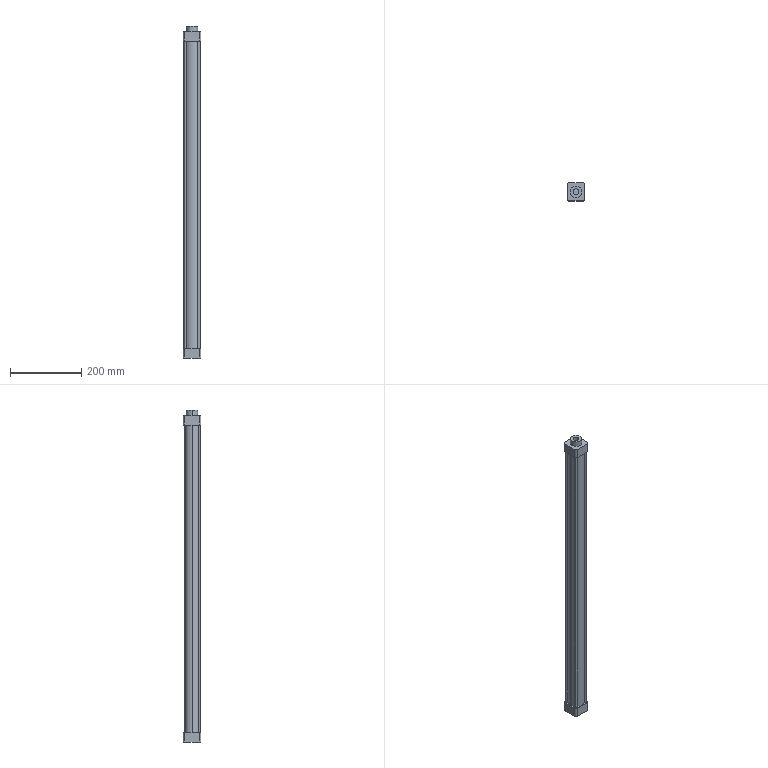Part | SolidWorks | features ICE 5, Extrusion 1, Fillet 1 | 1 solid | 39 faces | box 50 x 50 x 930 mm | volume 585630 mm3 | cylinder 24 | plane 15 | commonest cylinder face diameters 6 x8 10 x8 16 x2 32 x2 40 x2 46 x2
STEP:
#1=CARTESIAN_POINT('',(-15.5,-18.5,27.5));
#2=VERTEX_POINT('',#1);
#3=CARTESIAN_POINT('',(-21.5,-18.5,27.5));
#4=VERTEX_POINT('',#3);
#5=CARTESIAN_POINT('',(-18.5,-18.5,27.5));
#6=DIRECTION('',(0.,0.,1.));
#7=DIRECTION('',(1.,0.,0.));
#8=AXIS2_PLACEMENT_3D('',#5,#6,#7);
#9=CIRCLE('',#8,3.);
#10=EDGE_CURVE('',#2,#4,#9,.T.);
#11=ORIENTED_EDGE('',*,*,#10,.T.);
#12=CARTESIAN_POINT('',(-21.5,-18.5,887.5));
#13=VERTEX_POINT('',#12);
#14=CARTESIAN_POINT('',(-21.5,-18.5,-8.485));
#15=DIRECTION('',(0.,0.,1.));
#16=VECTOR('',#15,1000.);
#17=LINE('',#14,#16);
#18=EDGE_CURVE('',#4,#13,#17,.T.);
#19=ORIENTED_EDGE('',*,*,#18,.T.);
#20=CARTESIAN_POINT('',(-15.5,-18.5,887.5));
#21=VERTEX_POINT('',#20);
#22=CARTESIAN_POINT('',(-18.5,-18.5,887.5));
#23=DIRECTION('',(0.,0.,1.));
#24=DIRECTION('',(1.,0.,0.));
#25=AXIS2_PLACEMENT_3D('',#22,#23,#24);
#26=CIRCLE('',#25,3.);
#27=EDGE_CURVE('',#21,#13,#26,.T.);
#28=ORIENTED_EDGE('',*,*,#27,.F.);
#29=CARTESIAN_POINT('',(-15.5,-18.5,-8.485));
#30=DIRECTION('',(0.,0.,1.));
#31=VECTOR('',#30,1000.);
#32=LINE('',#29,#31);
#33=EDGE_CURVE('',#2,#21,#32,.T.);
#34=ORIENTED_EDGE('',*,*,#33,.F.);
#35=EDGE_LOOP('',(#11,#19,#28,#34));
#36=FACE_OUTER_BOUND('',#35,.T.);
#37=CARTESIAN_POINT('',(-18.5,-18.5,-8.485));
#38=DIRECTION('',(0.,0.,1.));
#39=DIRECTION('',(1.,0.,0.));
#40=AXIS2_PLACEMENT_3D('',#37,#38,#39);
#41=CYLINDRICAL_SURFACE('',#40,3.);
#42=ADVANCED_FACE('',(#36),#41,.T.);
#43=CARTESIAN_POINT('',(21.5,-18.5,27.5));
#44=VERTEX_POINT('',#43);
#45=CARTESIAN_POINT('',(15.5,-18.5,27.5));
#46=VERTEX_POINT('',#45);
#47=CARTESIAN_POINT('',(18.5,-18.5,27.5));
#48=DIRECTION('',(0.,0.,1.));
#49=DIRECTION('',(1.,0.,0.));
#50=AXIS2_PLACEMENT_3D('',#47,#48,#49);
#51=CIRCLE('',#50,3.);
#52=EDGE_CURVE('',#44,#46,#51,.T.);
#53=ORIENTED_EDGE('',*,*,#52,.T.);
#54=CARTESIAN_POINT('',(15.5,-18.5,887.5));
#55=VERTEX_POINT('',#54);
#56=CARTESIAN_POINT('',(15.5,-18.5,-8.485));
#57=DIRECTION('',(0.,0.,1.));
#58=VECTOR('',#57,1000.);
#59=LINE('',#56,#58);
#60=EDGE_CURVE('',#46,#55,#59,.T.);
#61=ORIENTED_EDGE('',*,*,#60,.T.);
#62=CARTESIAN_POINT('',(21.5,-18.5,887.5));
#63=VERTEX_POINT('',#62);
#64=CARTESIAN_POINT('',(18.5,-18.5,887.5));
#65=DIRECTION('',(0.,0.,1.));
#66=DIRECTION('',(1.,0.,0.));
#67=AXIS2_PLACEMENT_3D('',#64,#65,#66);
#68=CIRCLE('',#67,3.);
#69=EDGE_CURVE('',#63,#55,#68,.T.);
#70=ORIENTED_EDGE('',*,*,#69,.F.);
#71=CARTESIAN_POINT('',(21.5,-18.5,-8.485));
#72=DIRECTION('',(0.,0.,1.));
#73=VECTOR('',#72,1000.);
#74=LINE('',#71,#73);
#75=EDGE_CURVE('',#44,#63,#74,.T.);
#76=ORIENTED_EDGE('',*,*,#75,.F.);
#77=EDGE_LOOP('',(#53,#61,#70,#76));
#78=FACE_OUTER_BOUND('',#77,.T.);
#79=CARTESIAN_POINT('',(18.5,-18.5,-8.485));
#80=DIRECTION('',(0.,0.,1.));
#81=DIRECTION('',(1.,0.,0.));
#82=AXIS2_PLACEMENT_3D('',#79,#80,#81);
#83=CYLINDRICAL_SURFACE('',#82,3.);
#84=ADVANCED_FACE('',(#78),#83,.T.);
#85=CARTESIAN_POINT('',(21.5,18.5,27.5));
#86=VERTEX_POINT('',#85);
#87=CARTESIAN_POINT('',(15.5,18.5,27.5));
#88=VERTEX_POINT('',#87);
#89=CARTESIAN_POINT('',(18.5,18.5,27.5));
#90=DIRECTION('',(0.,0.,1.));
#91=DIRECTION('',(1.,0.,0.));
#92=AXIS2_PLACEMENT_3D('',#89,#90,#91);
#93=CIRCLE('',#92,3.);
#94=EDGE_CURVE('',#86,#88,#93,.T.);
#95=ORIENTED_EDGE('',*,*,#94,.T.);
#96=CARTESIAN_POINT('',(15.5,18.5,887.5));
#97=VERTEX_POINT('',#96);
#98=CARTESIAN_POINT('',(15.5,18.5,-8.485));
#99=DIRECTION('',(0.,0.,1.));
#100=VECTOR('',#99,1000.);
#101=LINE('',#98,#100);
#102=EDGE_CURVE('',#88,#97,#101,.T.);
#103=ORIENTED_EDGE('',*,*,#102,.T.);
#104=CARTESIAN_POINT('',(21.5,18.5,887.5));
#105=VERTEX_POINT('',#104);
#106=CARTESIAN_POINT('',(18.5,18.5,887.5));
#107=DIRECTION('',(0.,0.,1.));
#108=DIRECTION('',(1.,0.,0.));
#109=AXIS2_PLACEMENT_3D('',#106,#107,#108);
#110=CIRCLE('',#109,3.);
#111=EDGE_CURVE('',#105,#97,#110,.T.);
#112=ORIENTED_EDGE('',*,*,#111,.F.);
#113=CARTESIAN_POINT('',(21.5,18.5,-8.485));
#114=DIRECTION('',(0.,0.,1.));
#115=VECTOR('',#114,1000.);
#116=LINE('',#113,#115);
#117=EDGE_CURVE('',#86,#105,#116,.T.);
#118=ORIENTED_EDGE('',*,*,#117,.F.);
#119=EDGE_LOOP('',(#95,#103,#112,#118));
#120=FACE_OUTER_BOUND('',#119,.T.);
#121=CARTESIAN_POINT('',(18.5,18.5,-8.485));
#122=DIRECTION('',(0.,0.,1.));
#123=DIRECTION('',(1.,0.,0.));
#124=AXIS2_PLACEMENT_3D('',#121,#122,#123);
#125=CYLINDRICAL_SURFACE('',#124,3.);
#126=ADVANCED_FACE('',(#120),#125,.T.);
#127=CARTESIAN_POINT('',(-15.5,18.5,27.5));
#128=VERTEX_POINT('',#127);
#129=CARTESIAN_POINT('',(-21.5,18.5,27.5));
#130=VERTEX_POINT('',#129);
#131=CARTESIAN_POINT('',(-18.5,18.5,27.5));
#132=DIRECTION('',(0.,0.,1.));
#133=DIRECTION('',(1.,0.,0.));
#134=AXIS2_PLACEMENT_3D('',#131,#132,#133);
#135=CIRCLE('',#134,3.);
#136=EDGE_CURVE('',#128,#130,#135,.T.);
#137=ORIENTED_EDGE('',*,*,#136,.T.);
#138=CARTESIAN_POINT('',(-21.5,18.5,887.5));
#139=VERTEX_POINT('',#138);
#140=CARTESIAN_POINT('',(-21.5,18.5,-8.485));
#141=DIRECTION('',(0.,0.,1.));
#142=VECTOR('',#141,1000.);
#143=LINE('',#140,#142);
#144=EDGE_CURVE('',#130,#139,#143,.T.);
#145=ORIENTED_EDGE('',*,*,#144,.T.);
#146=CARTESIAN_POINT('',(-15.5,18.5,887.5));
#147=VERTEX_POINT('',#146);
#148=CARTESIAN_POINT('',(-18.5,18.5,887.5));
#149=DIRECTION('',(0.,0.,1.));
#150=DIRECTION('',(1.,0.,0.));
#151=AXIS2_PLACEMENT_3D('',#148,#149,#150);
#152=CIRCLE('',#151,3.);
#153=EDGE_CURVE('',#147,#139,#152,.T.);
#154=ORIENTED_EDGE('',*,*,#153,.F.);
#155=CARTESIAN_POINT('',(-15.5,18.5,-8.485));
#156=DIRECTION('',(0.,0.,1.));
#157=VECTOR('',#156,1000.);
#158=LINE('',#155,#157);
#159=EDGE_CURVE('',#128,#147,#158,.T.);
#160=ORIENTED_EDGE('',*,*,#159,.F.);
#161=EDGE_LOOP('',(#137,#145,#154,#160));
#162=FACE_OUTER_BOUND('',#161,.T.);
#163=CARTESIAN_POINT('',(-18.5,18.5,-8.485));
#164=DIRECTION('',(0.,0.,1.));
#165=DIRECTION('',(1.,0.,0.));
#166=AXIS2_PLACEMENT_3D('',#163,#164,#165);
#167=CYLINDRICAL_SURFACE('',#166,3.);
#168=ADVANCED_FACE('',(#162),#167,.T.);
#169=CARTESIAN_POINT('',(16.,0.,930.));
#170=VERTEX_POINT('',#169);
#171=CARTESIAN_POINT('',(-16.,0.,930.));
#172=VERTEX_POINT('',#171);
#173=CARTESIAN_POINT('',(0.,0.,930.));
#174=DIRECTION('',(0.,0.,1.));
#175=DIRECTION('',(1.,0.,0.));
#176=AXIS2_PLACEMENT_3D('',#173,#174,#175);
#177=CIRCLE('',#176,16.);
#178=EDGE_CURVE('',#170,#172,#177,.T.);
#179=ORIENTED_EDGE('',*,*,#178,.F.);
#180=CARTESIAN_POINT('',(16.,0.,915.));
#181=VERTEX_POINT('',#180);
#182=CARTESIAN_POINT('',(16.,0.,930.));
#183=DIRECTION('',(0.,0.,-1.));
#184=VECTOR('',#183,1000.);
#185=LINE('',#182,#184);
#186=EDGE_CURVE('',#170,#181,#185,.T.);
#187=ORIENTED_EDGE('',*,*,#186,.T.);
#188=CARTESIAN_POINT('',(-16.,0.,915.));
#189=VERTEX_POINT('',#188);
#190=CARTESIAN_POINT('',(0.,0.,915.));
#191=DIRECTION('',(0.,0.,1.));
#192=DIRECTION('',(1.,0.,0.));
#193=AXIS2_PLACEMENT_3D('',#190,#191,#192);
#194=CIRCLE('',#193,16.);
#195=EDGE_CURVE('',#181,#189,#194,.T.);
#196=ORIENTED_EDGE('',*,*,#195,.T.);
#197=CARTESIAN_POINT('',(-16.,0.,930.));
#198=DIRECTION('',(0.,0.,-1.));
#199=VECTOR('',#198,1000.);
#200=LINE('',#197,#199);
#201=EDGE_CURVE('',#172,#189,#200,.T.);
#202=ORIENTED_EDGE('',*,*,#201,.F.);
#203=EDGE_LOOP('',(#179,#187,#196,#202));
#204=FACE_OUTER_BOUND('',#203,.T.);
#205=CARTESIAN_POINT('',(0.,0.,930.));
#206=DIRECTION('',(0.,0.,-1.));
#207=DIRECTION('',(-1.,0.,0.));
#208=AXIS2_PLACEMENT_3D('',#205,#206,#207);
#209=CYLINDRICAL_SURFACE('',#208,16.);
#210=ADVANCED_FACE('',(#204),#209,.T.);
#211=CARTESIAN_POINT('',(23.,0.,887.5));
#212=VERTEX_POINT('',#211);
#213=CARTESIAN_POINT('',(-23.,0.,887.5));
#214=VERTEX_POINT('',#213);
#215=CARTESIAN_POINT('',(0.,0.,887.5));
#216=DIRECTION('',(0.,0.,1.));
#217=DIRECTION('',(1.,0.,0.));
#218=AXIS2_PLACEMENT_3D('',#215,#216,#217);
#219=CIRCLE('',#218,23.);
#220=EDGE_CURVE('',#212,#214,#219,.T.);
#221=ORIENTED_EDGE('',*,*,#220,.F.);
#222=CARTESIAN_POINT('',(23.,0.,27.5));
#223=VERTEX_POINT('',#222);
#224=CARTESIAN_POINT('',(23.,0.,887.5));
#225=DIRECTION('',(0.,0.,-1.));
#226=VECTOR('',#225,1000.);
#227=LINE('',#224,#226);
#228=EDGE_CURVE('',#212,#223,#227,.T.);
#229=ORIENTED_EDGE('',*,*,#228,.T.);
#230=CARTESIAN_POINT('',(-23.,0.,27.5));
#231=VERTEX_POINT('',#230);
#232=CARTESIAN_POINT('',(0.,0.,27.5));
#233=DIRECTION('',(0.,0.,1.));
#234=DIRECTION('',(1.,0.,0.));
#235=AXIS2_PLACEMENT_3D('',#232,#233,#234);
#236=CIRCLE('',#235,23.);
#237=EDGE_CURVE('',#223,#231,#236,.T.);
#238=ORIENTED_EDGE('',*,*,#237,.T.);
#239=CARTESIAN_POINT('',(-23.,0.,887.5));
#240=DIRECTION('',(0.,0.,-1.));
#241=VECTOR('',#240,1000.);
#242=LINE('',#239,#241);
#243=EDGE_CURVE('',#214,#231,#242,.T.);
#244=ORIENTED_EDGE('',*,*,#243,.F.);
#245=EDGE_LOOP('',(#221,#229,#238,#244));
#246=FACE_OUTER_BOUND('',#245,.T.);
#247=CARTESIAN_POINT('',(0.,0.,887.5));
#248=DIRECTION('',(0.,0.,-1.));
#249=DIRECTION('',(-1.,0.,0.));
#250=AXIS2_PLACEMENT_3D('',#247,#248,#249);
#251=CYLINDRICAL_SURFACE('',#250,23.);
#252=ADVANCED_FACE('',(#246),#251,.T.);
#253=CARTESIAN_POINT('',(-8.,0.,887.5));
#254=VERTEX_POINT('',#253);
#255=CARTESIAN_POINT('',(8.,0.,887.5));
#256=VERTEX_POINT('',#255);
#257=CARTESIAN_POINT('',(0.,0.,887.5));
#258=DIRECTION('',(0.,0.,1.));
#259=DIRECTION('',(1.,0.,0.));
#260=AXIS2_PLACEMENT_3D('',#257,#258,#259);
#261=CIRCLE('',#260,8.);
#262=EDGE_CURVE('',#254,#256,#261,.T.);
#263=ORIENTED_EDGE('',*,*,#262,.F.);
#264=CARTESIAN_POINT('',(-8.,0.,930.));
#265=VERTEX_POINT('',#264);
#266=CARTESIAN_POINT('',(-8.,0.,830.));
#267=DIRECTION('',(0.,0.,1.));
#268=VECTOR('',#267,1000.);
#269=LINE('',#266,#268);
#270=EDGE_CURVE('',#254,#265,#269,.T.);
#271=ORIENTED_EDGE('',*,*,#270,.T.);
#272=CARTESIAN_POINT('',(8.,0.,930.));
#273=VERTEX_POINT('',#272);
#274=CARTESIAN_POINT('',(0.,0.,930.));
#275=DIRECTION('',(0.,0.,1.));
#276=DIRECTION('',(1.,0.,0.));
#277=AXIS2_PLACEMENT_3D('',#274,#275,#276);
#278=CIRCLE('',#277,8.);
#279=EDGE_CURVE('',#265,#273,#278,.T.);
#280=ORIENTED_EDGE('',*,*,#279,.T.);
#281=CARTESIAN_POINT('',(8.,0.,830.));
#282=DIRECTION('',(0.,0.,1.));
#283=VECTOR('',#282,1000.);
#284=LINE('',#281,#283);
#285=EDGE_CURVE('',#256,#273,#284,.T.);
#286=ORIENTED_EDGE('',*,*,#285,.F.);
#287=EDGE_LOOP('',(#263,#271,#280,#286));
#288=FACE_OUTER_BOUND('',#287,.T.);
#289=CARTESIAN_POINT('',(0.,0.,830.));
#290=DIRECTION('',(0.,0.,1.));
#291=DIRECTION('',(1.,0.,0.));
#292=AXIS2_PLACEMENT_3D('',#289,#290,#291);
#293=CYLINDRICAL_SURFACE('',#292,8.);
#294=ADVANCED_FACE('',(#288),#293,.F.);
#295=CARTESIAN_POINT('',(-20.,0.,887.5));
#296=VERTEX_POINT('',#295);
#297=CARTESIAN_POINT('',(20.,0.,887.5));
#298=VERTEX_POINT('',#297);
#299=CARTESIAN_POINT('',(0.,0.,887.5));
#300=DIRECTION('',(0.,0.,1.));
#301=DIRECTION('',(1.,0.,0.));
#302=AXIS2_PLACEMENT_3D('',#299,#300,#301);
#303=CIRCLE('',#302,20.);
#304=EDGE_CURVE('',#296,#298,#303,.T.);
#305=ORIENTED_EDGE('',*,*,#304,.T.);
#306=CARTESIAN_POINT('',(20.,0.,27.5));
#307=VERTEX_POINT('',#306);
#308=CARTESIAN_POINT('',(20.,0.,887.5));
#309=DIRECTION('',(0.,0.,-1.));
#310=VECTOR('',#309,1000.);
#311=LINE('',#308,#310);
#312=EDGE_CURVE('',#298,#307,#311,.T.);
#313=ORIENTED_EDGE('',*,*,#312,.T.);
#314=CARTESIAN_POINT('',(-20.,0.,27.5));
#315=VERTEX_POINT('',#314);
#316=CARTESIAN_POINT('',(0.,0.,27.5));
#317=DIRECTION('',(0.,0.,-1.));
#318=DIRECTION('',(1.,0.,0.));
#319=AXIS2_PLACEMENT_3D('',#316,#317,#318);
#320=CIRCLE('',#319,20.);
#321=EDGE_CURVE('',#307,#315,#320,.T.);
#322=ORIENTED_EDGE('',*,*,#321,.T.);
#323=CARTESIAN_POINT('',(-20.,0.,887.5));
#324=DIRECTION('',(0.,0.,-1.));
#325=VECTOR('',#324,1000.);
#326=LINE('',#323,#325);
#327=EDGE_CURVE('',#296,#315,#326,.T.);
#328=ORIENTED_EDGE('',*,*,#327,.F.);
#329=EDGE_LOOP('',(#305,#313,#322,#328));
#330=FACE_OUTER_BOUND('',#329,.T.);
#331=CARTESIAN_POINT('',(0.,0.,887.5));
#332=DIRECTION('',(0.,0.,-1.));
#333=DIRECTION('',(-1.,0.,0.));
#334=AXIS2_PLACEMENT_3D('',#331,#332,#333);
#335=CYLINDRICAL_SURFACE('',#334,20.);
#336=ADVANCED_FACE('',(#330),#335,.F.);
#337=CARTESIAN_POINT('',(0.,0.,27.5));
#338=DIRECTION('',(0.,0.,-1.));
#339=DIRECTION('',(1.,0.,0.));
#340=AXIS2_PLACEMENT_3D('',#337,#338,#339);
#341=CIRCLE('',#340,20.);
#342=EDGE_CURVE('',#315,#307,#341,.T.);
#343=ORIENTED_EDGE('',*,*,#342,.F.);
#344=ORIENTED_EDGE('',*,*,#321,.F.);
#345=EDGE_LOOP('',(#343,#344));
#346=FACE_OUTER_BOUND('',#345,.T.);
#347=CARTESIAN_POINT('',(0.,0.,27.5));
#348=DIRECTION('',(0.,0.,1.));
#349=DIRECTION('',(1.,0.,0.));
#350=AXIS2_PLACEMENT_3D('',#347,#348,#349);
#351=PLANE('',#350);
#352=ADVANCED_FACE('',(#346),#351,.T.);
#353=ORIENTED_EDGE('',*,*,#312,.F.);
#354=CARTESIAN_POINT('',(0.,0.,887.5));
#355=DIRECTION('',(0.,0.,1.));
#356=DIRECTION('',(1.,0.,0.));
#357=AXIS2_PLACEMENT_3D('',#354,#355,#356);
#358=CIRCLE('',#357,20.);
#359=EDGE_CURVE('',#298,#296,#358,.T.);
#360=ORIENTED_EDGE('',*,*,#359,.T.);
#361=ORIENTED_EDGE('',*,*,#327,.T.);
#362=ORIENTED_EDGE('',*,*,#342,.T.);
#363=EDGE_LOOP('',(#353,#360,#361,#362));
#364=FACE_OUTER_BOUND('',#363,.T.);
#365=CARTESIAN_POINT('',(0.,0.,887.5));
#366=DIRECTION('',(0.,0.,-1.));
#367=DIRECTION('',(-1.,0.,0.));
#368=AXIS2_PLACEMENT_3D('',#365,#366,#367);
#369=CYLINDRICAL_SURFACE('',#368,20.);
#370=ADVANCED_FACE('',(#364),#369,.F.);
#371=CARTESIAN_POINT('',(0.,0.,887.5));
#372=DIRECTION('',(0.,0.,1.));
#373=DIRECTION('',(1.,0.,0.));
#374=AXIS2_PLACEMENT_3D('',#371,#372,#373);
#375=CIRCLE('',#374,8.);
#376=EDGE_CURVE('',#256,#254,#375,.T.);
#377=ORIENTED_EDGE('',*,*,#376,.T.);
#378=ORIENTED_EDGE('',*,*,#262,.T.);
#379=EDGE_LOOP('',(#377,#378));
#380=FACE_BOUND('',#379,.T.);
#381=ORIENTED_EDGE('',*,*,#304,.F.);
#382=ORIENTED_EDGE('',*,*,#359,.F.);
#383=EDGE_LOOP('',(#381,#382));
#384=FACE_OUTER_BOUND('',#383,.T.);
#385=CARTESIAN_POINT('',(0.,0.,887.5));
#386=DIRECTION('',(0.,0.,1.));
#387=DIRECTION('',(1.,0.,0.));
#388=AXIS2_PLACEMENT_3D('',#385,#386,#387);
#389=PLANE('',#388);
#390=ADVANCED_FACE('',(#380,#384),#389,.F.);
#391=ORIENTED_EDGE('',*,*,#270,.F.);
#392=ORIENTED_EDGE('',*,*,#376,.F.);
#393=ORIENTED_EDGE('',*,*,#285,.T.);
#394=CARTESIAN_POINT('',(0.,0.,930.));
#395=DIRECTION('',(0.,0.,1.));
#396=DIRECTION('',(1.,0.,0.));
#397=AXIS2_PLACEMENT_3D('',#394,#395,#396);
#398=CIRCLE('',#397,8.);
#399=EDGE_CURVE('',#273,#265,#398,.T.);
#400=ORIENTED_EDGE('',*,*,#399,.T.);
#401=EDGE_LOOP('',(#391,#392,#393,#400));
#402=FACE_OUTER_BOUND('',#401,.T.);
#403=CARTESIAN_POINT('',(0.,0.,830.));
#404=DIRECTION('',(0.,0.,1.));
#405=DIRECTION('',(1.,0.,0.));
#406=AXIS2_PLACEMENT_3D('',#403,#404,#405);
#407=CYLINDRICAL_SURFACE('',#406,8.);
#408=ADVANCED_FACE('',(#402),#407,.F.);
#409=CARTESIAN_POINT('',(25.,-20.,27.5));
#410=VERTEX_POINT('',#409);
#411=CARTESIAN_POINT('',(25.,20.,27.5));
#412=VERTEX_POINT('',#411);
#413=CARTESIAN_POINT('',(25.,25.,27.5));
#414=DIRECTION('',(0.,1.,0.));
#415=VECTOR('',#414,1000.);
#416=LINE('',#413,#415);
#417=EDGE_CURVE('',#410,#412,#416,.T.);
#418=ORIENTED_EDGE('',*,*,#417,.F.);
#419=CARTESIAN_POINT('',(25.,-20.,0.));
#420=VERTEX_POINT('',#419);
#421=CARTESIAN_POINT('',(25.,-20.,27.5));
#422=DIRECTION('',(0.,0.,-1.));
#423=VECTOR('',#422,1000.);
#424=LINE('',#421,#423);
#425=EDGE_CURVE('',#410,#420,#424,.T.);
#426=ORIENTED_EDGE('',*,*,#425,.T.);
#427=CARTESIAN_POINT('',(25.,20.,0.));
#428=VERTEX_POINT('',#427);
#429=CARTESIAN_POINT('',(25.,25.,0.));
#430=DIRECTION('',(0.,1.,0.));
#431=VECTOR('',#430,1000.);
#432=LINE('',#429,#431);
#433=EDGE_CURVE('',#420,#428,#432,.T.);
#434=ORIENTED_EDGE('',*,*,#433,.T.);
#435=CARTESIAN_POINT('',(25.,20.,27.5));
#436=DIRECTION('',(0.,0.,1.));
#437=VECTOR('',#436,1000.);
#438=LINE('',#435,#437);
#439=EDGE_CURVE('',#428,#412,#438,.T.);
#440=ORIENTED_EDGE('',*,*,#439,.T.);
#441=EDGE_LOOP('',(#418,#426,#434,#440));
#442=FACE_OUTER_BOUND('',#441,.T.);
#443=CARTESIAN_POINT('',(25.,25.,27.5));
#444=DIRECTION('',(-1.,0.,0.));
#445=DIRECTION('',(0.,0.,1.));
#446=AXIS2_PLACEMENT_3D('',#443,#444,#445);
#447=PLANE('',#446);
#448=ADVANCED_FACE('',(#442),#447,.F.);
#449=CARTESIAN_POINT('',(20.,25.,0.));
#450=VERTEX_POINT('',#449);
#451=CARTESIAN_POINT('',(-20.,25.,0.));
#452=VERTEX_POINT('',#451);
#453=CARTESIAN_POINT('',(-25.,25.,0.));
#454=DIRECTION('',(-1.,0.,0.));
#455=VECTOR('',#454,1000.);
#456=LINE('',#453,#455);
#457=EDGE_CURVE('',#450,#452,#456,.T.);
#458=ORIENTED_EDGE('',*,*,#457,.T.);
#459=CARTESIAN_POINT('',(-20.,25.,27.5));
#460=VERTEX_POINT('',#459);
#461=CARTESIAN_POINT('',(-20.,25.,27.5));
#462=DIRECTION('',(0.,0.,1.));
#463=VECTOR('',#462,1000.);
#464=LINE('',#461,#463);
#465=EDGE_CURVE('',#452,#460,#464,.T.);
#466=ORIENTED_EDGE('',*,*,#465,.T.);
#467=CARTESIAN_POINT('',(20.,25.,27.5));
#468=VERTEX_POINT('',#467);
#469=CARTESIAN_POINT('',(-25.,25.,27.5));
#470=DIRECTION('',(-1.,0.,0.));
#471=VECTOR('',#470,1000.);
#472=LINE('',#469,#471);
#473=EDGE_CURVE('',#468,#460,#472,.T.);
#474=ORIENTED_EDGE('',*,*,#473,.F.);
#475=CARTESIAN_POINT('',(20.,25.,27.5));
#476=DIRECTION('',(0.,0.,-1.));
#477=VECTOR('',#476,1000.);
#478=LINE('',#475,#477);
#479=EDGE_CURVE('',#468,#450,#478,.T.);
#480=ORIENTED_EDGE('',*,*,#479,.T.);
#481=EDGE_LOOP('',(#458,#466,#474,#480));
#482=FACE_OUTER_BOUND('',#481,.T.);
#483=CARTESIAN_POINT('',(-25.,25.,27.5));
#484=DIRECTION('',(0.,-1.,0.));
#485=DIRECTION('',(0.,0.,-1.));
#486=AXIS2_PLACEMENT_3D('',#483,#484,#485);
#487=PLANE('',#486);
#488=ADVANCED_FACE('',(#482),#487,.F.);
#489=CARTESIAN_POINT('',(-25.,20.,0.));
#490=VERTEX_POINT('',#489);
#491=CARTESIAN_POINT('',(-25.,-20.,0.));
#492=VERTEX_POINT('',#491);
#493=CARTESIAN_POINT('',(-25.,25.,0.));
#494=DIRECTION('',(0.,-1.,0.));
#495=VECTOR('',#494,1000.);
#496=LINE('',#493,#495);
#497=EDGE_CURVE('',#490,#492,#496,.T.);
#498=ORIENTED_EDGE('',*,*,#497,.T.);
#499=CARTESIAN_POINT('',(-25.,-20.,27.5));
#500=VERTEX_POINT('',#499);
#501=CARTESIAN_POINT('',(-25.,-20.,27.5));
#502=DIRECTION('',(0.,0.,1.));
#503=VECTOR('',#502,1000.);
#504=LINE('',#501,#503);
#505=EDGE_CURVE('',#492,#500,#504,.T.);
#506=ORIENTED_EDGE('',*,*,#505,.T.);
#507=CARTESIAN_POINT('',(-25.,20.,27.5));
#508=VERTEX_POINT('',#507);
#509=CARTESIAN_POINT('',(-25.,25.,27.5));
#510=DIRECTION('',(0.,-1.,0.));
#511=VECTOR('',#510,1000.);
#512=LINE('',#509,#511);
#513=EDGE_CURVE('',#508,#500,#512,.T.);
#514=ORIENTED_EDGE('',*,*,#513,.F.);
#515=CARTESIAN_POINT('',(-25.,20.,27.5));
#516=DIRECTION('',(0.,0.,-1.));
#517=VECTOR('',#516,1000.);
#518=LINE('',#515,#517);
#519=EDGE_CURVE('',#508,#490,#518,.T.);
#520=ORIENTED_EDGE('',*,*,#519,.T.);
#521=EDGE_LOOP('',(#498,#506,#514,#520));
#522=FACE_OUTER_BOUND('',#521,.T.);
#523=CARTESIAN_POINT('',(-25.,25.,27.5));
#524=DIRECTION('',(1.,0.,0.));
#525=DIRECTION('',(0.,1.,0.));
#526=AXIS2_PLACEMENT_3D('',#523,#524,#525);
#527=PLANE('',#526);
#528=ADVANCED_FACE('',(#522),#527,.F.);
#529=CARTESIAN_POINT('',(-20.,-25.,27.5));
#530=VERTEX_POINT('',#529);
#531=CARTESIAN_POINT('',(20.,-25.,27.5));
#532=VERTEX_POINT('',#531);
#533=CARTESIAN_POINT('',(-25.,-25.,27.5));
#534=DIRECTION('',(1.,0.,0.));
#535=VECTOR('',#534,1000.);
#536=LINE('',#533,#535);
#537=EDGE_CURVE('',#530,#532,#536,.T.);
#538=ORIENTED_EDGE('',*,*,#537,.F.);
#539=CARTESIAN_POINT('',(-20.,-25.,0.));
#540=VERTEX_POINT('',#539);
#541=CARTESIAN_POINT('',(-20.,-25.,27.5));
#542=DIRECTION('',(0.,0.,-1.));
#543=VECTOR('',#542,1000.);
#544=LINE('',#541,#543);
#545=EDGE_CURVE('',#530,#540,#544,.T.);
#546=ORIENTED_EDGE('',*,*,#545,.T.);
#547=CARTESIAN_POINT('',(20.,-25.,0.));
#548=VERTEX_POINT('',#547);
#549=CARTESIAN_POINT('',(-25.,-25.,0.));
#550=DIRECTION('',(1.,0.,0.));
#551=VECTOR('',#550,1000.);
#552=LINE('',#549,#551);
#553=EDGE_CURVE('',#540,#548,#552,.T.);
#554=ORIENTED_EDGE('',*,*,#553,.T.);
#555=CARTESIAN_POINT('',(20.,-25.,27.5));
#556=DIRECTION('',(0.,0.,1.));
#557=VECTOR('',#556,1000.);
#558=LINE('',#555,#557);
#559=EDGE_CURVE('',#548,#532,#558,.T.);
#560=ORIENTED_EDGE('',*,*,#559,.T.);
#561=EDGE_LOOP('',(#538,#546,#554,#560));
#562=FACE_OUTER_BOUND('',#561,.T.);
#563=CARTESIAN_POINT('',(-25.,-25.,27.5));
#564=DIRECTION('',(0.,1.,0.));
#565=DIRECTION('',(0.,0.,1.));
#566=AXIS2_PLACEMENT_3D('',#563,#564,#565);
#567=PLANE('',#566);
#568=ADVANCED_FACE('',(#562),#567,.F.);
#569=ORIENTED_EDGE('',*,*,#10,.F.);
#570=CARTESIAN_POINT('',(-18.5,-18.5,27.5));
#571=DIRECTION('',(0.,0.,1.));
#572=DIRECTION('',(1.,0.,0.));
#573=AXIS2_PLACEMENT_3D('',#570,#571,#572);
#574=CIRCLE('',#573,3.);
#575=EDGE_CURVE('',#4,#2,#574,.T.);
#576=ORIENTED_EDGE('',*,*,#575,.F.);
#577=EDGE_LOOP('',(#569,#576));
#578=FACE_BOUND('',#577,.T.);
#579=ORIENTED_EDGE('',*,*,#52,.F.);
#580=CARTESIAN_POINT('',(18.5,-18.5,27.5));
#581=DIRECTION('',(0.,0.,1.));
#582=DIRECTION('',(1.,0.,0.));
#583=AXIS2_PLACEMENT_3D('',#580,#581,#582);
#584=CIRCLE('',#583,3.);
#585=EDGE_CURVE('',#46,#44,#584,.T.);
#586=ORIENTED_EDGE('',*,*,#585,.F.);
#587=EDGE_LOOP('',(#579,#586));
#588=FACE_BOUND('',#587,.T.);
#589=ORIENTED_EDGE('',*,*,#94,.F.);
#590=CARTESIAN_POINT('',(18.5,18.5,27.5));
#591=DIRECTION('',(0.,0.,1.));
#592=DIRECTION('',(1.,0.,0.));
#593=AXIS2_PLACEMENT_3D('',#590,#591,#592);
#594=CIRCLE('',#593,3.);
#595=EDGE_CURVE('',#88,#86,#594,.T.);
#596=ORIENTED_EDGE('',*,*,#595,.F.);
#597=EDGE_LOOP('',(#589,#596));
#598=FACE_BOUND('',#597,.T.);
#599=ORIENTED_EDGE('',*,*,#136,.F.);
#600=CARTESIAN_POINT('',(-18.5,18.5,27.5));
#601=DIRECTION('',(0.,0.,1.));
#602=DIRECTION('',(1.,0.,0.));
#603=AXIS2_PLACEMENT_3D('',#600,#601,#602);
#604=CIRCLE('',#603,3.);
#605=EDGE_CURVE('',#130,#128,#604,.T.);
#606=ORIENTED_EDGE('',*,*,#605,.F.);
#607=EDGE_LOOP('',(#599,#606));
#608=FACE_BOUND('',#607,.T.);
#609=CARTESIAN_POINT('',(0.,0.,27.5));
#610=DIRECTION('',(0.,0.,1.));
#611=DIRECTION('',(1.,0.,0.));
#612=AXIS2_PLACEMENT_3D('',#609,#610,#611);
#613=CIRCLE('',#612,23.);
#614=EDGE_CURVE('',#231,#223,#613,.T.);
#615=ORIENTED_EDGE('',*,*,#614,.F.);
#616=ORIENTED_EDGE('',*,*,#237,.F.);
#617=EDGE_LOOP('',(#615,#616));
#618=FACE_BOUND('',#617,.T.);
#619=ORIENTED_EDGE('',*,*,#513,.T.);
#620=CARTESIAN_POINT('',(-20.,-20.,27.5));
#621=DIRECTION('',(0.,0.,1.));
#622=DIRECTION('',(1.,0.,0.));
#623=AXIS2_PLACEMENT_3D('',#620,#621,#622);
#624=CIRCLE('',#623,5.);
#625=EDGE_CURVE('',#500,#530,#624,.T.);
#626=ORIENTED_EDGE('',*,*,#625,.T.);
#627=ORIENTED_EDGE('',*,*,#537,.T.);
#628=CARTESIAN_POINT('',(20.,-20.,27.5));
#629=DIRECTION('',(0.,0.,1.));
#630=DIRECTION('',(1.,0.,0.));
#631=AXIS2_PLACEMENT_3D('',#628,#629,#630);
#632=CIRCLE('',#631,5.);
#633=EDGE_CURVE('',#532,#410,#632,.T.);
#634=ORIENTED_EDGE('',*,*,#633,.T.);
#635=ORIENTED_EDGE('',*,*,#417,.T.);
#636=CARTESIAN_POINT('',(20.,20.,27.5));
#637=DIRECTION('',(0.,0.,1.));
#638=DIRECTION('',(1.,0.,0.));
#639=AXIS2_PLACEMENT_3D('',#636,#637,#638);
#640=CIRCLE('',#639,5.);
#641=EDGE_CURVE('',#412,#468,#640,.T.);
#642=ORIENTED_EDGE('',*,*,#641,.T.);
#643=ORIENTED_EDGE('',*,*,#473,.T.);
#644=CARTESIAN_POINT('',(-20.,20.,27.5));
#645=DIRECTION('',(0.,0.,1.));
#646=DIRECTION('',(1.,0.,0.));
#647=AXIS2_PLACEMENT_3D('',#644,#645,#646);
#648=CIRCLE('',#647,5.);
#649=EDGE_CURVE('',#460,#508,#648,.T.);
#650=ORIENTED_EDGE('',*,*,#649,.T.);
#651=EDGE_LOOP('',(#619,#626,#627,#634,#635,#642,#643,#650));
#652=FACE_OUTER_BOUND('',#651,.T.);
#653=CARTESIAN_POINT('',(0.,0.,27.5));
#654=DIRECTION('',(0.,0.,1.));
#655=DIRECTION('',(1.,0.,0.));
#656=AXIS2_PLACEMENT_3D('',#653,#654,#655);
#657=PLANE('',#656);
#658=ADVANCED_FACE('',(#578,#588,#598,#608,#618,#652),#657,.T.);
#659=ORIENTED_EDGE('',*,*,#553,.F.);
#660=CARTESIAN_POINT('',(-20.,-20.,0.));
#661=DIRECTION('',(0.,0.,-1.));
#662=DIRECTION('',(1.,0.,0.));
#663=AXIS2_PLACEMENT_3D('',#660,#661,#662);
#664=CIRCLE('',#663,5.);
#665=EDGE_CURVE('',#540,#492,#664,.T.);
#666=ORIENTED_EDGE('',*,*,#665,.T.);
#667=ORIENTED_EDGE('',*,*,#497,.F.);
#668=CARTESIAN_POINT('',(-20.,20.,0.));
#669=DIRECTION('',(0.,0.,-1.));
#670=DIRECTION('',(1.,0.,0.));
#671=AXIS2_PLACEMENT_3D('',#668,#669,#670);
#672=CIRCLE('',#671,5.);
#673=EDGE_CURVE('',#490,#452,#672,.T.);
#674=ORIENTED_EDGE('',*,*,#673,.T.);
#675=ORIENTED_EDGE('',*,*,#457,.F.);
#676=CARTESIAN_POINT('',(20.,20.,0.));
#677=DIRECTION('',(0.,0.,-1.));
#678=DIRECTION('',(1.,0.,0.));
#679=AXIS2_PLACEMENT_3D('',#676,#677,#678);
#680=CIRCLE('',#679,5.);
#681=EDGE_CURVE('',#450,#428,#680,.T.);
#682=ORIENTED_EDGE('',*,*,#681,.T.);
#683=ORIENTED_EDGE('',*,*,#433,.F.);
#684=CARTESIAN_POINT('',(20.,-20.,0.));
#685=DIRECTION('',(0.,0.,-1.));
#686=DIRECTION('',(1.,0.,0.));
#687=AXIS2_PLACEMENT_3D('',#684,#685,#686);
#688=CIRCLE('',#687,5.);
#689=EDGE_CURVE('',#420,#548,#688,.T.);
#690=ORIENTED_EDGE('',*,*,#689,.T.);
#691=EDGE_LOOP('',(#659,#666,#667,#674,#675,#682,#683,#690));
#692=FACE_OUTER_BOUND('',#691,.T.);
#693=CARTESIAN_POINT('',(0.,0.,0.));
#694=DIRECTION('',(0.,0.,1.));
#695=DIRECTION('',(1.,0.,0.));
#696=AXIS2_PLACEMENT_3D('',#693,#694,#695);
#697=PLANE('',#696);
#698=ADVANCED_FACE('',(#692),#697,.F.);
#699=ORIENTED_EDGE('',*,*,#228,.F.);
#700=CARTESIAN_POINT('',(0.,0.,887.5));
#701=DIRECTION('',(0.,0.,1.));
#702=DIRECTION('',(1.,0.,0.));
#703=AXIS2_PLACEMENT_3D('',#700,#701,#702);
#704=CIRCLE('',#703,23.);
#705=EDGE_CURVE('',#214,#212,#704,.T.);
#706=ORIENTED_EDGE('',*,*,#705,.F.);
#707=ORIENTED_EDGE('',*,*,#243,.T.);
#708=ORIENTED_EDGE('',*,*,#614,.T.);
#709=EDGE_LOOP('',(#699,#706,#707,#708));
#710=FACE_OUTER_BOUND('',#709,.T.);
#711=CARTESIAN_POINT('',(0.,0.,887.5));
#712=DIRECTION('',(0.,0.,-1.));
#713=DIRECTION('',(-1.,0.,0.));
#714=AXIS2_PLACEMENT_3D('',#711,#712,#713);
#715=CYLINDRICAL_SURFACE('',#714,23.);
#716=ADVANCED_FACE('',(#710),#715,.T.);
#717=CARTESIAN_POINT('',(25.,-20.,915.));
#718=VERTEX_POINT('',#717);
#719=CARTESIAN_POINT('',(25.,20.,915.));
#720=VERTEX_POINT('',#719);
#721=CARTESIAN_POINT('',(25.,25.,915.));
#722=DIRECTION('',(0.,1.,0.));
#723=VECTOR('',#722,1000.);
#724=LINE('',#721,#723);
#725=EDGE_CURVE('',#718,#720,#724,.T.);
#726=ORIENTED_EDGE('',*,*,#725,.F.);
#727=CARTESIAN_POINT('',(25.,-20.,887.5));
#728=VERTEX_POINT('',#727);
#729=CARTESIAN_POINT('',(25.,-20.,915.));
#730=DIRECTION('',(0.,0.,-1.));
#731=VECTOR('',#730,1000.);
#732=LINE('',#729,#731);
#733=EDGE_CURVE('',#718,#728,#732,.T.);
#734=ORIENTED_EDGE('',*,*,#733,.T.);
#735=CARTESIAN_POINT('',(25.,20.,887.5));
#736=VERTEX_POINT('',#735);
#737=CARTESIAN_POINT('',(25.,25.,887.5));
#738=DIRECTION('',(0.,1.,0.));
#739=VECTOR('',#738,1000.);
#740=LINE('',#737,#739);
#741=EDGE_CURVE('',#728,#736,#740,.T.);
#742=ORIENTED_EDGE('',*,*,#741,.T.);
#743=CARTESIAN_POINT('',(25.,20.,915.));
#744=DIRECTION('',(0.,0.,1.));
#745=VECTOR('',#744,1000.);
#746=LINE('',#743,#745);
#747=EDGE_CURVE('',#736,#720,#746,.T.);
#748=ORIENTED_EDGE('',*,*,#747,.T.);
#749=EDGE_LOOP('',(#726,#734,#742,#748));
#750=FACE_OUTER_BOUND('',#749,.T.);
#751=CARTESIAN_POINT('',(25.,25.,915.));
#752=DIRECTION('',(-1.,0.,0.));
#753=DIRECTION('',(0.,-1.,0.));
#754=AXIS2_PLACEMENT_3D('',#751,#752,#753);
#755=PLANE('',#754);
#756=ADVANCED_FACE('',(#750),#755,.F.);
#757=CARTESIAN_POINT('',(20.,25.,887.5));
#758=VERTEX_POINT('',#757);
#759=CARTESIAN_POINT('',(-20.,25.,887.5));
#760=VERTEX_POINT('',#759);
#761=CARTESIAN_POINT('',(-25.,25.,887.5));
#762=DIRECTION('',(-1.,0.,0.));
#763=VECTOR('',#762,1000.);
#764=LINE('',#761,#763);
#765=EDGE_CURVE('',#758,#760,#764,.T.);
#766=ORIENTED_EDGE('',*,*,#765,.T.);
#767=CARTESIAN_POINT('',(-20.,25.,915.));
#768=VERTEX_POINT('',#767);
#769=CARTESIAN_POINT('',(-20.,25.,915.));
#770=DIRECTION('',(0.,0.,1.));
#771=VECTOR('',#770,1000.);
#772=LINE('',#769,#771);
#773=EDGE_CURVE('',#760,#768,#772,.T.);
#774=ORIENTED_EDGE('',*,*,#773,.T.);
#775=CARTESIAN_POINT('',(20.,25.,915.));
#776=VERTEX_POINT('',#775);
#777=CARTESIAN_POINT('',(-25.,25.,915.));
#778=DIRECTION('',(-1.,0.,0.));
#779=VECTOR('',#778,1000.);
#780=LINE('',#777,#779);
#781=EDGE_CURVE('',#776,#768,#780,.T.);
#782=ORIENTED_EDGE('',*,*,#781,.F.);
#783=CARTESIAN_POINT('',(20.,25.,915.));
#784=DIRECTION('',(0.,0.,-1.));
#785=VECTOR('',#784,1000.);
#786=LINE('',#783,#785);
#787=EDGE_CURVE('',#776,#758,#786,.T.);
#788=ORIENTED_EDGE('',*,*,#787,.T.);
#789=EDGE_LOOP('',(#766,#774,#782,#788));
#790=FACE_OUTER_BOUND('',#789,.T.);
#791=CARTESIAN_POINT('',(-25.,25.,915.));
#792=DIRECTION('',(0.,-1.,0.));
#793=DIRECTION('',(0.,0.,-1.));
#794=AXIS2_PLACEMENT_3D('',#791,#792,#793);
#795=PLANE('',#794);
#796=ADVANCED_FACE('',(#790),#795,.F.);
#797=CARTESIAN_POINT('',(-25.,20.,887.5));
#798=VERTEX_POINT('',#797);
#799=CARTESIAN_POINT('',(-25.,-20.,887.5));
#800=VERTEX_POINT('',#799);
#801=CARTESIAN_POINT('',(-25.,25.,887.5));
#802=DIRECTION('',(0.,-1.,0.));
#803=VECTOR('',#802,1000.);
#804=LINE('',#801,#803);
#805=EDGE_CURVE('',#798,#800,#804,.T.);
#806=ORIENTED_EDGE('',*,*,#805,.T.);
#807=CARTESIAN_POINT('',(-25.,-20.,915.));
#808=VERTEX_POINT('',#807);
#809=CARTESIAN_POINT('',(-25.,-20.,915.));
#810=DIRECTION('',(0.,0.,1.));
#811=VECTOR('',#810,1000.);
#812=LINE('',#809,#811);
#813=EDGE_CURVE('',#800,#808,#812,.T.);
#814=ORIENTED_EDGE('',*,*,#813,.T.);
#815=CARTESIAN_POINT('',(-25.,20.,915.));
#816=VERTEX_POINT('',#815);
#817=CARTESIAN_POINT('',(-25.,25.,915.));
#818=DIRECTION('',(0.,-1.,0.));
#819=VECTOR('',#818,1000.);
#820=LINE('',#817,#819);
#821=EDGE_CURVE('',#816,#808,#820,.T.);
#822=ORIENTED_EDGE('',*,*,#821,.F.);
#823=CARTESIAN_POINT('',(-25.,20.,915.));
#824=DIRECTION('',(0.,0.,-1.));
#825=VECTOR('',#824,1000.);
#826=LINE('',#823,#825);
#827=EDGE_CURVE('',#816,#798,#826,.T.);
#828=ORIENTED_EDGE('',*,*,#827,.T.);
#829=EDGE_LOOP('',(#806,#814,#822,#828));
#830=FACE_OUTER_BOUND('',#829,.T.);
#831=CARTESIAN_POINT('',(-25.,25.,915.));
#832=DIRECTION('',(1.,0.,0.));
#833=DIRECTION('',(0.,1.,0.));
#834=AXIS2_PLACEMENT_3D('',#831,#832,#833);
#835=PLANE('',#834);
#836=ADVANCED_FACE('',(#830),#835,.F.);
#837=CARTESIAN_POINT('',(-20.,-25.,915.));
#838=VERTEX_POINT('',#837);
#839=CARTESIAN_POINT('',(20.,-25.,915.));
#840=VERTEX_POINT('',#839);
#841=CARTESIAN_POINT('',(-25.,-25.,915.));
#842=DIRECTION('',(1.,0.,0.));
#843=VECTOR('',#842,1000.);
#844=LINE('',#841,#843);
#845=EDGE_CURVE('',#838,#840,#844,.T.);
#846=ORIENTED_EDGE('',*,*,#845,.F.);
#847=CARTESIAN_POINT('',(-20.,-25.,887.5));
#848=VERTEX_POINT('',#847);
#849=CARTESIAN_POINT('',(-20.,-25.,915.));
#850=DIRECTION('',(0.,0.,-1.));
#851=VECTOR('',#850,1000.);
#852=LINE('',#849,#851);
#853=EDGE_CURVE('',#838,#848,#852,.T.);
#854=ORIENTED_EDGE('',*,*,#853,.T.);
#855=CARTESIAN_POINT('',(20.,-25.,887.5));
#856=VERTEX_POINT('',#855);
#857=CARTESIAN_POINT('',(-25.,-25.,887.5));
#858=DIRECTION('',(1.,0.,0.));
#859=VECTOR('',#858,1000.);
#860=LINE('',#857,#859);
#861=EDGE_CURVE('',#848,#856,#860,.T.);
#862=ORIENTED_EDGE('',*,*,#861,.T.);
#863=CARTESIAN_POINT('',(20.,-25.,915.));
#864=DIRECTION('',(0.,0.,1.));
#865=VECTOR('',#864,1000.);
#866=LINE('',#863,#865);
#867=EDGE_CURVE('',#856,#840,#866,.T.);
#868=ORIENTED_EDGE('',*,*,#867,.T.);
#869=EDGE_LOOP('',(#846,#854,#862,#868));
#870=FACE_OUTER_BOUND('',#869,.T.);
#871=CARTESIAN_POINT('',(-25.,-25.,915.));
#872=DIRECTION('',(0.,1.,0.));
#873=DIRECTION('',(0.,0.,1.));
#874=AXIS2_PLACEMENT_3D('',#871,#872,#873);
#875=PLANE('',#874);
#876=ADVANCED_FACE('',(#870),#875,.F.);
#877=CARTESIAN_POINT('',(0.,0.,915.));
#878=DIRECTION('',(0.,0.,1.));
#879=DIRECTION('',(1.,0.,0.));
#880=AXIS2_PLACEMENT_3D('',#877,#878,#879);
#881=CIRCLE('',#880,16.);
#882=EDGE_CURVE('',#189,#181,#881,.T.);
#883=ORIENTED_EDGE('',*,*,#882,.F.);
#884=ORIENTED_EDGE('',*,*,#195,.F.);
#885=EDGE_LOOP('',(#883,#884));
#886=FACE_BOUND('',#885,.T.);
#887=ORIENTED_EDGE('',*,*,#821,.T.);
#888=CARTESIAN_POINT('',(-20.,-20.,915.));
#889=DIRECTION('',(0.,0.,1.));
#890=DIRECTION('',(1.,0.,0.));
#891=AXIS2_PLACEMENT_3D('',#888,#889,#890);
#892=CIRCLE('',#891,5.);
#893=EDGE_CURVE('',#808,#838,#892,.T.);
#894=ORIENTED_EDGE('',*,*,#893,.T.);
#895=ORIENTED_EDGE('',*,*,#845,.T.);
#896=CARTESIAN_POINT('',(20.,-20.,915.));
#897=DIRECTION('',(0.,0.,1.));
#898=DIRECTION('',(1.,0.,0.));
#899=AXIS2_PLACEMENT_3D('',#896,#897,#898);
#900=CIRCLE('',#899,5.);
#901=EDGE_CURVE('',#840,#718,#900,.T.);
#902=ORIENTED_EDGE('',*,*,#901,.T.);
#903=ORIENTED_EDGE('',*,*,#725,.T.);
#904=CARTESIAN_POINT('',(20.,20.,915.));
#905=DIRECTION('',(0.,0.,1.));
#906=DIRECTION('',(1.,0.,0.));
#907=AXIS2_PLACEMENT_3D('',#904,#905,#906);
#908=CIRCLE('',#907,5.);
#909=EDGE_CURVE('',#720,#776,#908,.T.);
#910=ORIENTED_EDGE('',*,*,#909,.T.);
#911=ORIENTED_EDGE('',*,*,#781,.T.);
#912=CARTESIAN_POINT('',(-20.,20.,915.));
#913=DIRECTION('',(0.,0.,1.));
#914=DIRECTION('',(1.,0.,0.));
#915=AXIS2_PLACEMENT_3D('',#912,#913,#914);
#916=CIRCLE('',#915,5.);
#917=EDGE_CURVE('',#768,#816,#916,.T.);
#918=ORIENTED_EDGE('',*,*,#917,.T.);
#919=EDGE_LOOP('',(#887,#894,#895,#902,#903,#910,#911,#918));
#920=FACE_OUTER_BOUND('',#919,.T.);
#921=CARTESIAN_POINT('',(0.,0.,915.));
#922=DIRECTION('',(0.,0.,1.));
#923=DIRECTION('',(1.,0.,0.));
#924=AXIS2_PLACEMENT_3D('',#921,#922,#923);
#925=PLANE('',#924);
#926=ADVANCED_FACE('',(#886,#920),#925,.T.);
#927=ORIENTED_EDGE('',*,*,#27,.T.);
#928=CARTESIAN_POINT('',(-18.5,-18.5,887.5));
#929=DIRECTION('',(0.,0.,1.));
#930=DIRECTION('',(1.,0.,0.));
#931=AXIS2_PLACEMENT_3D('',#928,#929,#930);
#932=CIRCLE('',#931,3.);
#933=EDGE_CURVE('',#13,#21,#932,.T.);
#934=ORIENTED_EDGE('',*,*,#933,.T.);
#935=EDGE_LOOP('',(#927,#934));
#936=FACE_BOUND('',#935,.T.);
#937=ORIENTED_EDGE('',*,*,#69,.T.);
#938=CARTESIAN_POINT('',(18.5,-18.5,887.5));
#939=DIRECTION('',(0.,0.,1.));
#940=DIRECTION('',(1.,0.,0.));
#941=AXIS2_PLACEMENT_3D('',#938,#939,#940);
#942=CIRCLE('',#941,3.);
#943=EDGE_CURVE('',#55,#63,#942,.T.);
#944=ORIENTED_EDGE('',*,*,#943,.T.);
#945=EDGE_LOOP('',(#937,#944));
#946=FACE_BOUND('',#945,.T.);
#947=ORIENTED_EDGE('',*,*,#111,.T.);
#948=CARTESIAN_POINT('',(18.5,18.5,887.5));
#949=DIRECTION('',(0.,0.,1.));
#950=DIRECTION('',(1.,0.,0.));
#951=AXIS2_PLACEMENT_3D('',#948,#949,#950);
#952=CIRCLE('',#951,3.);
#953=EDGE_CURVE('',#97,#105,#952,.T.);
#954=ORIENTED_EDGE('',*,*,#953,.T.);
#955=EDGE_LOOP('',(#947,#954));
#956=FACE_BOUND('',#955,.T.);
#957=ORIENTED_EDGE('',*,*,#153,.T.);
#958=CARTESIAN_POINT('',(-18.5,18.5,887.5));
#959=DIRECTION('',(0.,0.,1.));
#960=DIRECTION('',(1.,0.,0.));
#961=AXIS2_PLACEMENT_3D('',#958,#959,#960);
#962=CIRCLE('',#961,3.);
#963=EDGE_CURVE('',#139,#147,#962,.T.);
#964=ORIENTED_EDGE('',*,*,#963,.T.);
#965=EDGE_LOOP('',(#957,#964));
#966=FACE_BOUND('',#965,.T.);
#967=ORIENTED_EDGE('',*,*,#705,.T.);
#968=ORIENTED_EDGE('',*,*,#220,.T.);
#969=EDGE_LOOP('',(#967,#968));
#970=FACE_BOUND('',#969,.T.);
#971=ORIENTED_EDGE('',*,*,#861,.F.);
#972=CARTESIAN_POINT('',(-20.,-20.,887.5));
#973=DIRECTION('',(0.,0.,-1.));
#974=DIRECTION('',(1.,0.,0.));
#975=AXIS2_PLACEMENT_3D('',#972,#973,#974);
#976=CIRCLE('',#975,5.);
#977=EDGE_CURVE('',#848,#800,#976,.T.);
#978=ORIENTED_EDGE('',*,*,#977,.T.);
#979=ORIENTED_EDGE('',*,*,#805,.F.);
#980=CARTESIAN_POINT('',(-20.,20.,887.5));
#981=DIRECTION('',(0.,0.,-1.));
#982=DIRECTION('',(1.,0.,0.));
#983=AXIS2_PLACEMENT_3D('',#980,#981,#982);
#984=CIRCLE('',#983,5.);
#985=EDGE_CURVE('',#798,#760,#984,.T.);
#986=ORIENTED_EDGE('',*,*,#985,.T.);
#987=ORIENTED_EDGE('',*,*,#765,.F.);
#988=CARTESIAN_POINT('',(20.,20.,887.5));
#989=DIRECTION('',(0.,0.,-1.));
#990=DIRECTION('',(1.,0.,0.));
#991=AXIS2_PLACEMENT_3D('',#988,#989,#990);
#992=CIRCLE('',#991,5.);
#993=EDGE_CURVE('',#758,#736,#992,.T.);
#994=ORIENTED_EDGE('',*,*,#993,.T.);
#995=ORIENTED_EDGE('',*,*,#741,.F.);
#996=CARTESIAN_POINT('',(20.,-20.,887.5));
#997=DIRECTION('',(0.,0.,-1.));
#998=DIRECTION('',(1.,0.,0.));
#999=AXIS2_PLACEMENT_3D('',#996,#997,#998);
#1000=CIRCLE('',#999,5.);
#1001=EDGE_CURVE('',#728,#856,#1000,.T.);
#1002=ORIENTED_EDGE('',*,*,#1001,.T.);
#1003=EDGE_LOOP('',(#971,#978,#979,#986,#987,#994,#995,#1002));
#1004=FACE_OUTER_BOUND('',#1003,.T.);
#1005=CARTESIAN_POINT('',(0.,0.,887.5));
#1006=DIRECTION('',(0.,0.,1.));
#1007=DIRECTION('',(1.,0.,0.));
#1008=AXIS2_PLACEMENT_3D('',#1005,#1006,#1007);
#1009=PLANE('',#1008);
#1010=ADVANCED_FACE('',(#936,#946,#956,#966,#970,#1004),#1009,.F.);
#1011=ORIENTED_EDGE('',*,*,#186,.F.);
#1012=CARTESIAN_POINT('',(0.,0.,930.));
#1013=DIRECTION('',(0.,0.,1.));
#1014=DIRECTION('',(1.,0.,0.));
#1015=AXIS2_PLACEMENT_3D('',#1012,#1013,#1014);
#1016=CIRCLE('',#1015,16.);
#1017=EDGE_CURVE('',#172,#170,#1016,.T.);
#1018=ORIENTED_EDGE('',*,*,#1017,.F.);
#1019=ORIENTED_EDGE('',*,*,#201,.T.);
#1020=ORIENTED_EDGE('',*,*,#882,.T.);
#1021=EDGE_LOOP('',(#1011,#1018,#1019,#1020));
#1022=FACE_OUTER_BOUND('',#1021,.T.);
#1023=CARTESIAN_POINT('',(0.,0.,930.));
#1024=DIRECTION('',(0.,0.,-1.));
#1025=DIRECTION('',(-1.,0.,0.));
#1026=AXIS2_PLACEMENT_3D('',#1023,#1024,#1025);
#1027=CYLINDRICAL_SURFACE('',#1026,16.);
#1028=ADVANCED_FACE('',(#1022),#1027,.T.);
#1029=ORIENTED_EDGE('',*,*,#399,.F.);
#1030=ORIENTED_EDGE('',*,*,#279,.F.);
#1031=EDGE_LOOP('',(#1029,#1030));
#1032=FACE_BOUND('',#1031,.T.);
#1033=ORIENTED_EDGE('',*,*,#1017,.T.);
#1034=ORIENTED_EDGE('',*,*,#178,.T.);
#1035=EDGE_LOOP('',(#1033,#1034));
#1036=FACE_OUTER_BOUND('',#1035,.T.);
#1037=CARTESIAN_POINT('',(0.,0.,930.));
#1038=DIRECTION('',(0.,0.,1.));
#1039=DIRECTION('',(1.,0.,0.));
#1040=AXIS2_PLACEMENT_3D('',#1037,#1038,#1039);
#1041=PLANE('',#1040);
#1042=ADVANCED_FACE('',(#1032,#1036),#1041,.T.);
#1043=ORIENTED_EDGE('',*,*,#144,.F.);
#1044=ORIENTED_EDGE('',*,*,#605,.T.);
#1045=ORIENTED_EDGE('',*,*,#159,.T.);
#1046=ORIENTED_EDGE('',*,*,#963,.F.);
#1047=EDGE_LOOP('',(#1043,#1044,#1045,#1046));
#1048=FACE_OUTER_BOUND('',#1047,.T.);
#1049=CARTESIAN_POINT('',(-18.5,18.5,-8.485));
#1050=DIRECTION('',(0.,0.,1.));
#1051=DIRECTION('',(1.,0.,0.));
#1052=AXIS2_PLACEMENT_3D('',#1049,#1050,#1051);
#1053=CYLINDRICAL_SURFACE('',#1052,3.);
#1054=ADVANCED_FACE('',(#1048),#1053,.T.);
#1055=ORIENTED_EDGE('',*,*,#102,.F.);
#1056=ORIENTED_EDGE('',*,*,#595,.T.);
#1057=ORIENTED_EDGE('',*,*,#117,.T.);
#1058=ORIENTED_EDGE('',*,*,#953,.F.);
#1059=EDGE_LOOP('',(#1055,#1056,#1057,#1058));
#1060=FACE_OUTER_BOUND('',#1059,.T.);
#1061=CARTESIAN_POINT('',(18.5,18.5,-8.485));
#1062=DIRECTION('',(0.,0.,1.));
#1063=DIRECTION('',(1.,0.,0.));
#1064=AXIS2_PLACEMENT_3D('',#1061,#1062,#1063);
#1065=CYLINDRICAL_SURFACE('',#1064,3.);
#1066=ADVANCED_FACE('',(#1060),#1065,.T.);
#1067=ORIENTED_EDGE('',*,*,#60,.F.);
#1068=ORIENTED_EDGE('',*,*,#585,.T.);
#1069=ORIENTED_EDGE('',*,*,#75,.T.);
#1070=ORIENTED_EDGE('',*,*,#943,.F.);
#1071=EDGE_LOOP('',(#1067,#1068,#1069,#1070));
#1072=FACE_OUTER_BOUND('',#1071,.T.);
#1073=CARTESIAN_POINT('',(18.5,-18.5,-8.485));
#1074=DIRECTION('',(0.,0.,1.));
#1075=DIRECTION('',(1.,0.,0.));
#1076=AXIS2_PLACEMENT_3D('',#1073,#1074,#1075);
#1077=CYLINDRICAL_SURFACE('',#1076,3.);
#1078=ADVANCED_FACE('',(#1072),#1077,.T.);
#1079=ORIENTED_EDGE('',*,*,#18,.F.);
#1080=ORIENTED_EDGE('',*,*,#575,.T.);
#1081=ORIENTED_EDGE('',*,*,#33,.T.);
#1082=ORIENTED_EDGE('',*,*,#933,.F.);
#1083=EDGE_LOOP('',(#1079,#1080,#1081,#1082));
#1084=FACE_OUTER_BOUND('',#1083,.T.);
#1085=CARTESIAN_POINT('',(-18.5,-18.5,-8.485));
#1086=DIRECTION('',(0.,0.,1.));
#1087=DIRECTION('',(1.,0.,0.));
#1088=AXIS2_PLACEMENT_3D('',#1085,#1086,#1087);
#1089=CYLINDRICAL_SURFACE('',#1088,3.);
#1090=ADVANCED_FACE('',(#1084),#1089,.T.);
#1091=ORIENTED_EDGE('',*,*,#625,.F.);
#1092=ORIENTED_EDGE('',*,*,#505,.F.);
#1093=ORIENTED_EDGE('',*,*,#665,.F.);
#1094=ORIENTED_EDGE('',*,*,#545,.F.);
#1095=EDGE_LOOP('',(#1091,#1092,#1093,#1094));
#1096=FACE_OUTER_BOUND('',#1095,.T.);
#1097=CARTESIAN_POINT('',(-20.,-20.,27.5));
#1098=DIRECTION('',(0.,0.,-1.));
#1099=DIRECTION('',(-1.,0.,0.));
#1100=AXIS2_PLACEMENT_3D('',#1097,#1098,#1099);
#1101=CYLINDRICAL_SURFACE('',#1100,5.);
#1102=ADVANCED_FACE('',(#1096),#1101,.T.);
#1103=ORIENTED_EDGE('',*,*,#893,.F.);
#1104=ORIENTED_EDGE('',*,*,#813,.F.);
#1105=ORIENTED_EDGE('',*,*,#977,.F.);
#1106=ORIENTED_EDGE('',*,*,#853,.F.);
#1107=EDGE_LOOP('',(#1103,#1104,#1105,#1106));
#1108=FACE_OUTER_BOUND('',#1107,.T.);
#1109=CARTESIAN_POINT('',(-20.,-20.,915.));
#1110=DIRECTION('',(0.,0.,-1.));
#1111=DIRECTION('',(-1.,0.,0.));
#1112=AXIS2_PLACEMENT_3D('',#1109,#1110,#1111);
#1113=CYLINDRICAL_SURFACE('',#1112,5.);
#1114=ADVANCED_FACE('',(#1108),#1113,.T.);
#1115=ORIENTED_EDGE('',*,*,#633,.F.);
#1116=ORIENTED_EDGE('',*,*,#559,.F.);
#1117=ORIENTED_EDGE('',*,*,#689,.F.);
#1118=ORIENTED_EDGE('',*,*,#425,.F.);
#1119=EDGE_LOOP('',(#1115,#1116,#1117,#1118));
#1120=FACE_OUTER_BOUND('',#1119,.T.);
#1121=CARTESIAN_POINT('',(20.,-20.,27.5));
#1122=DIRECTION('',(0.,0.,-1.));
#1123=DIRECTION('',(-1.,0.,0.));
#1124=AXIS2_PLACEMENT_3D('',#1121,#1122,#1123);
#1125=CYLINDRICAL_SURFACE('',#1124,5.);
#1126=ADVANCED_FACE('',(#1120),#1125,.T.);
#1127=ORIENTED_EDGE('',*,*,#901,.F.);
#1128=ORIENTED_EDGE('',*,*,#867,.F.);
#1129=ORIENTED_EDGE('',*,*,#1001,.F.);
#1130=ORIENTED_EDGE('',*,*,#733,.F.);
#1131=EDGE_LOOP('',(#1127,#1128,#1129,#1130));
#1132=FACE_OUTER_BOUND('',#1131,.T.);
#1133=CARTESIAN_POINT('',(20.,-20.,915.));
#1134=DIRECTION('',(0.,0.,-1.));
#1135=DIRECTION('',(-1.,0.,0.));
#1136=AXIS2_PLACEMENT_3D('',#1133,#1134,#1135);
#1137=CYLINDRICAL_SURFACE('',#1136,5.);
#1138=ADVANCED_FACE('',(#1132),#1137,.T.);
#1139=ORIENTED_EDGE('',*,*,#917,.F.);
#1140=ORIENTED_EDGE('',*,*,#773,.F.);
#1141=ORIENTED_EDGE('',*,*,#985,.F.);
#1142=ORIENTED_EDGE('',*,*,#827,.F.);
#1143=EDGE_LOOP('',(#1139,#1140,#1141,#1142));
#1144=FACE_OUTER_BOUND('',#1143,.T.);
#1145=CARTESIAN_POINT('',(-20.,20.,915.));
#1146=DIRECTION('',(0.,0.,-1.));
#1147=DIRECTION('',(-1.,0.,0.));
#1148=AXIS2_PLACEMENT_3D('',#1145,#1146,#1147);
#1149=CYLINDRICAL_SURFACE('',#1148,5.);
#1150=ADVANCED_FACE('',(#1144),#1149,.T.);
#1151=ORIENTED_EDGE('',*,*,#649,.F.);
#1152=ORIENTED_EDGE('',*,*,#465,.F.);
#1153=ORIENTED_EDGE('',*,*,#673,.F.);
#1154=ORIENTED_EDGE('',*,*,#519,.F.);
#1155=EDGE_LOOP('',(#1151,#1152,#1153,#1154));
#1156=FACE_OUTER_BOUND('',#1155,.T.);
#1157=CARTESIAN_POINT('',(-20.,20.,27.5));
#1158=DIRECTION('',(0.,0.,-1.));
#1159=DIRECTION('',(-1.,0.,0.));
#1160=AXIS2_PLACEMENT_3D('',#1157,#1158,#1159);
#1161=CYLINDRICAL_SURFACE('',#1160,5.);
#1162=ADVANCED_FACE('',(#1156),#1161,.T.);
#1163=ORIENTED_EDGE('',*,*,#641,.F.);
#1164=ORIENTED_EDGE('',*,*,#439,.F.);
#1165=ORIENTED_EDGE('',*,*,#681,.F.);
#1166=ORIENTED_EDGE('',*,*,#479,.F.);
#1167=EDGE_LOOP('',(#1163,#1164,#1165,#1166));
#1168=FACE_OUTER_BOUND('',#1167,.T.);
#1169=CARTESIAN_POINT('',(20.,20.,27.5));
#1170=DIRECTION('',(0.,0.,-1.));
#1171=DIRECTION('',(-1.,0.,0.));
#1172=AXIS2_PLACEMENT_3D('',#1169,#1170,#1171);
#1173=CYLINDRICAL_SURFACE('',#1172,5.);
#1174=ADVANCED_FACE('',(#1168),#1173,.T.);
#1175=ORIENTED_EDGE('',*,*,#909,.F.);
#1176=ORIENTED_EDGE('',*,*,#747,.F.);
#1177=ORIENTED_EDGE('',*,*,#993,.F.);
#1178=ORIENTED_EDGE('',*,*,#787,.F.);
#1179=EDGE_LOOP('',(#1175,#1176,#1177,#1178));
#1180=FACE_OUTER_BOUND('',#1179,.T.);
#1181=CARTESIAN_POINT('',(20.,20.,915.));
#1182=DIRECTION('',(0.,0.,-1.));
#1183=DIRECTION('',(-1.,0.,0.));
#1184=AXIS2_PLACEMENT_3D('',#1181,#1182,#1183);
#1185=CYLINDRICAL_SURFACE('',#1184,5.);
#1186=ADVANCED_FACE('',(#1180),#1185,.T.);
#1187=CLOSED_SHELL('',(#42,#84,#126,#168,#210,#252,#294,#336,#352,#370,#390,#408,#448,#488,#528,#568,#658,#698,#716,#756,#796,#836,#876,#926,#1010,#1028,#1042,#1054,#1066,#1078,#1090,#1102,#1114,#1126,#1138,#1150,#1162,#1174,#1186));
#1188=MANIFOLD_SOLID_BREP('',#1187);
#1189=CARTESIAN_POINT('',(0.,0.,0.));
#1190=DIRECTION('',(0.,0.,1.));
#1191=DIRECTION('',(1.,0.,0.));
#1192=AXIS2_PLACEMENT_3D('',#1189,#1190,#1191);
#1193=(LENGTH_UNIT()NAMED_UNIT(*)SI_UNIT(.MILLI.,.METRE.));
#1194=UNCERTAINTY_MEASURE_WITH_UNIT(LENGTH_MEASURE(0.00001),#1193,'','');
#1195=(NAMED_UNIT(*)PLANE_ANGLE_UNIT()SI_UNIT($,.RADIAN.));
#1196=(NAMED_UNIT(*)SI_UNIT($,.STERADIAN.)SOLID_ANGLE_UNIT());
#1197=(GEOMETRIC_REPRESENTATION_CONTEXT(3)GLOBAL_UNCERTAINTY_ASSIGNED_CONTEXT((#1194))GLOBAL_UNIT_ASSIGNED_CONTEXT((#1193,#1195,#1196))REPRESENTATION_CONTEXT('',''));
#1198=ADVANCED_BREP_SHAPE_REPRESENTATION('',(#1188,#1192),#1197);